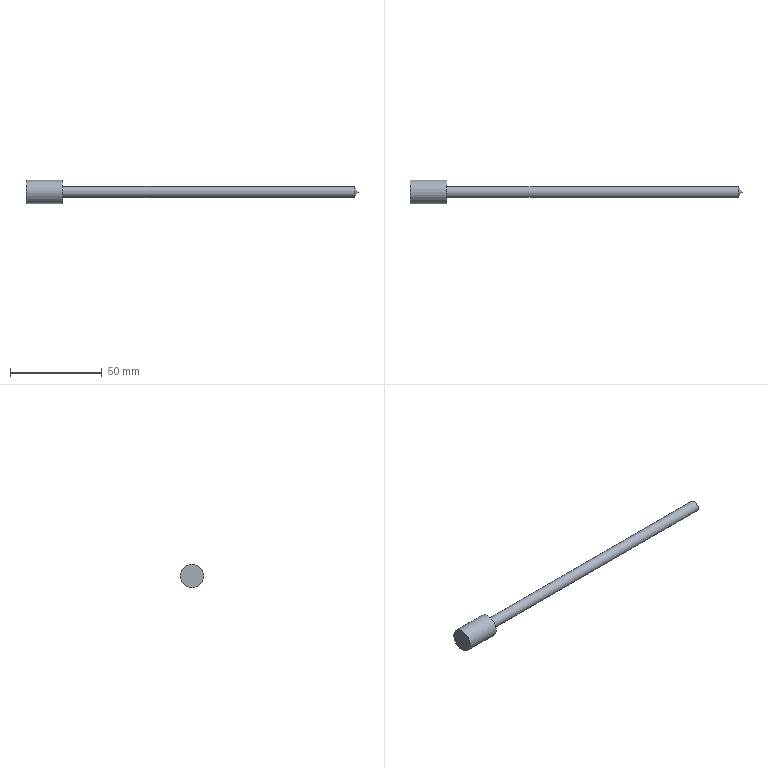Part | NX | features solid 2 | 1 solid | 5 faces | box 180.803 x 12.7 x 12.7 mm | volume 7046 mm3 | plane 2 | cylinder 2 | cone 1 | commonest cylinder face diameters 6 x1 12.7 x1
STEP:
#1=CARTESIAN_POINT('',(-155.,-50.,-84.));
#2=VERTEX_POINT('',#1);
#3=CARTESIAN_POINT('',(-155.,-50.,-87.));
#4=DIRECTION('',(-1.,0.,0.));
#5=DIRECTION('',(0.,0.,1.));
#6=AXIS2_PLACEMENT_3D('',#3,#4,#5);
#7=CIRCLE('',#6,3.);
#8=EDGE_CURVE('',#2,#2,#7,.T.);
#9=ORIENTED_EDGE('',*,*,#8,.T.);
#10=EDGE_LOOP('',(#9));
#11=FACE_BOUND('',#10,.T.);
#12=CARTESIAN_POINT('',(-155.,-50.,-80.65));
#13=VERTEX_POINT('',#12);
#14=CARTESIAN_POINT('',(-155.,-50.,-87.));
#15=DIRECTION('',(1.,0.,0.));
#16=DIRECTION('',(0.,0.,1.));
#17=AXIS2_PLACEMENT_3D('',#14,#15,#16);
#18=CIRCLE('',#17,6.35);
#19=EDGE_CURVE('',#13,#13,#18,.T.);
#20=ORIENTED_EDGE('',*,*,#19,.T.);
#21=EDGE_LOOP('',(#20));
#22=FACE_BOUND('',#21,.T.);
#23=CARTESIAN_POINT('',(-155.,-50.,-87.));
#24=DIRECTION('',(1.,0.,0.));
#25=DIRECTION('',(0.,0.,1.));
#26=AXIS2_PLACEMENT_3D('',#23,#24,#25);
#27=PLANE('',#26);
#28=ADVANCED_FACE('',(#11,#22),#27,.T.);
#29=CARTESIAN_POINT('',(-175.,-50.,-80.65));
#30=VERTEX_POINT('',#29);
#31=CARTESIAN_POINT('',(-175.,-50.,-87.));
#32=DIRECTION('',(-1.,0.,0.));
#33=DIRECTION('',(0.,0.,1.));
#34=AXIS2_PLACEMENT_3D('',#31,#32,#33);
#35=CIRCLE('',#34,6.35);
#36=EDGE_CURVE('',#30,#30,#35,.T.);
#37=ORIENTED_EDGE('',*,*,#36,.T.);
#38=EDGE_LOOP('',(#37));
#39=FACE_BOUND('',#38,.T.);
#40=CARTESIAN_POINT('',(-175.,-50.,-87.));
#41=DIRECTION('',(-1.,0.,0.));
#42=DIRECTION('',(0.,0.,-1.));
#43=AXIS2_PLACEMENT_3D('',#40,#41,#42);
#44=PLANE('',#43);
#45=ADVANCED_FACE('',(#39),#44,.T.);
#46=ORIENTED_EDGE('',*,*,#19,.F.);
#47=EDGE_LOOP('',(#46));
#48=FACE_BOUND('',#47,.T.);
#49=ORIENTED_EDGE('',*,*,#36,.F.);
#50=EDGE_LOOP('',(#49));
#51=FACE_BOUND('',#50,.T.);
#52=CARTESIAN_POINT('',(-175.,-50.,-87.));
#53=DIRECTION('',(1.,0.,0.));
#54=DIRECTION('',(0.,0.,1.));
#55=AXIS2_PLACEMENT_3D('',#52,#53,#54);
#56=CYLINDRICAL_SURFACE('',#55,6.35);
#57=ADVANCED_FACE('',(#48,#51),#56,.T.);
#58=ORIENTED_EDGE('',*,*,#8,.F.);
#59=EDGE_LOOP('',(#58));
#60=FACE_BOUND('',#59,.T.);
#61=CARTESIAN_POINT('',(4.,-50.,-84.));
#62=VERTEX_POINT('',#61);
#63=CARTESIAN_POINT('',(4.,-50.,-87.));
#64=DIRECTION('',(-1.,0.,0.));
#65=DIRECTION('',(0.,0.,1.));
#66=AXIS2_PLACEMENT_3D('',#63,#64,#65);
#67=CIRCLE('',#66,3.);
#68=EDGE_CURVE('',#62,#62,#67,.T.);
#69=ORIENTED_EDGE('',*,*,#68,.T.);
#70=EDGE_LOOP('',(#69));
#71=FACE_BOUND('',#70,.T.);
#72=CARTESIAN_POINT('',(-175.,-50.,-87.));
#73=DIRECTION('',(1.,0.,0.));
#74=DIRECTION('',(0.,0.,1.));
#75=AXIS2_PLACEMENT_3D('',#72,#73,#74);
#76=CYLINDRICAL_SURFACE('',#75,3.);
#77=ADVANCED_FACE('',(#60,#71),#76,.T.);
#78=ORIENTED_EDGE('',*,*,#68,.F.);
#79=EDGE_LOOP('',(#78));
#80=FACE_BOUND('',#79,.T.);
#81=CARTESIAN_POINT('',(5.803,-50.,-87.));
#82=VERTEX_POINT('',#81);
#83=VERTEX_LOOP('',#82);
#84=FACE_BOUND('',#83,.T.);
#85=CARTESIAN_POINT('',(5.803,-50.,-87.));
#86=DIRECTION('',(-1.,0.,0.));
#87=DIRECTION('',(0.,0.,1.));
#88=AXIS2_PLACEMENT_3D('',#85,#86,#87);
#89=CONICAL_SURFACE('',#88,0.,1.03);
#90=ADVANCED_FACE('',(#80,#84),#89,.T.);
#91=CLOSED_SHELL('',(#28,#45,#57,#77,#90));
#92=MANIFOLD_SOLID_BREP('',#91);
#93=(LENGTH_UNIT()NAMED_UNIT(*)SI_UNIT(.MILLI.,.METRE.));
#94=UNCERTAINTY_MEASURE_WITH_UNIT(LENGTH_MEASURE(0.00001),#93,'','');
#95=(NAMED_UNIT(*)PLANE_ANGLE_UNIT()SI_UNIT($,.RADIAN.));
#96=(NAMED_UNIT(*)SI_UNIT($,.STERADIAN.)SOLID_ANGLE_UNIT());
#97=(GEOMETRIC_REPRESENTATION_CONTEXT(3)GLOBAL_UNCERTAINTY_ASSIGNED_CONTEXT((#94))GLOBAL_UNIT_ASSIGNED_CONTEXT((#93,#95,#96))REPRESENTATION_CONTEXT('',''));
#98=ADVANCED_BREP_SHAPE_REPRESENTATION('',(#92),#97);